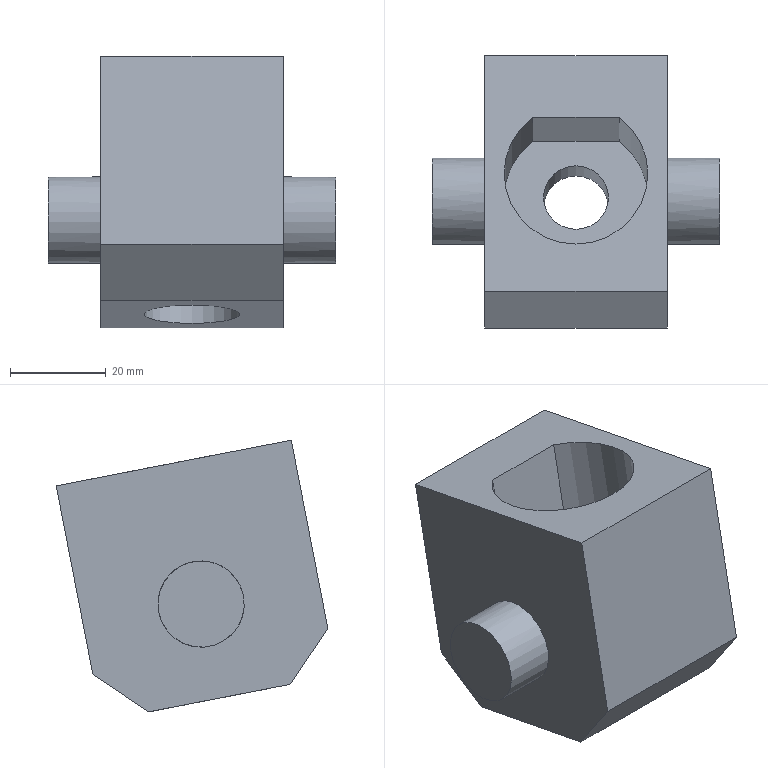Part | STEP file | solid 85 | 1 solid | 18 faces | box 60 x 56.714 x 56.714 mm | volume 73718 mm3 | plane 13 | cylinder 5 | commonest cylinder face diameters 18 x2 13.5 x1 20 x1 30 x1